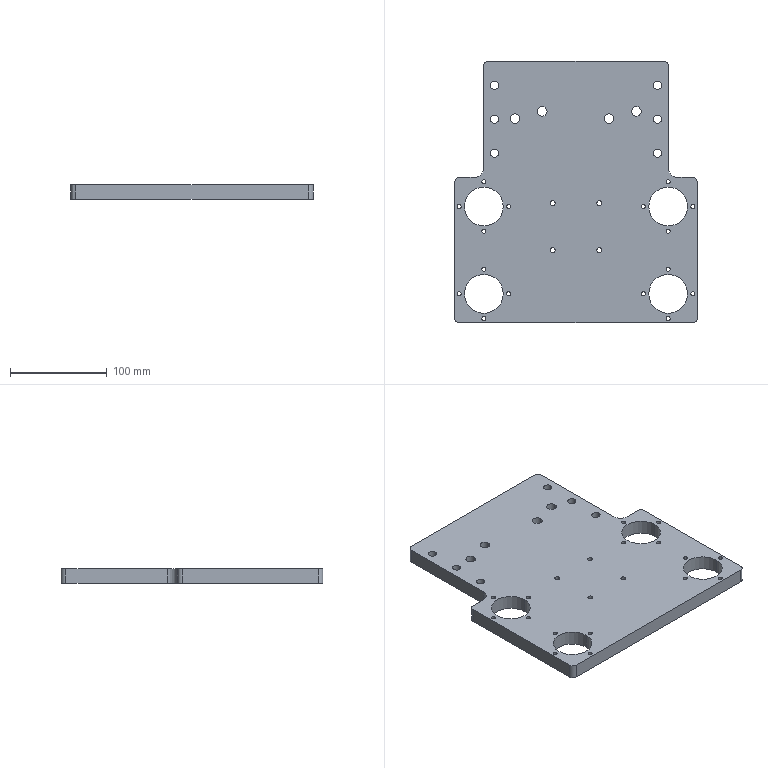Part | STEP file | 03-28 press moving plate | 1 solid | 86 faces | box 250 x 270 x 15 mm | volume 814940 mm3 | cylinder 76 | plane 10 | commonest cylinder face diameters 4.2 x32 10 x14 8.5 x12 5 x8 40 x8 20 x2